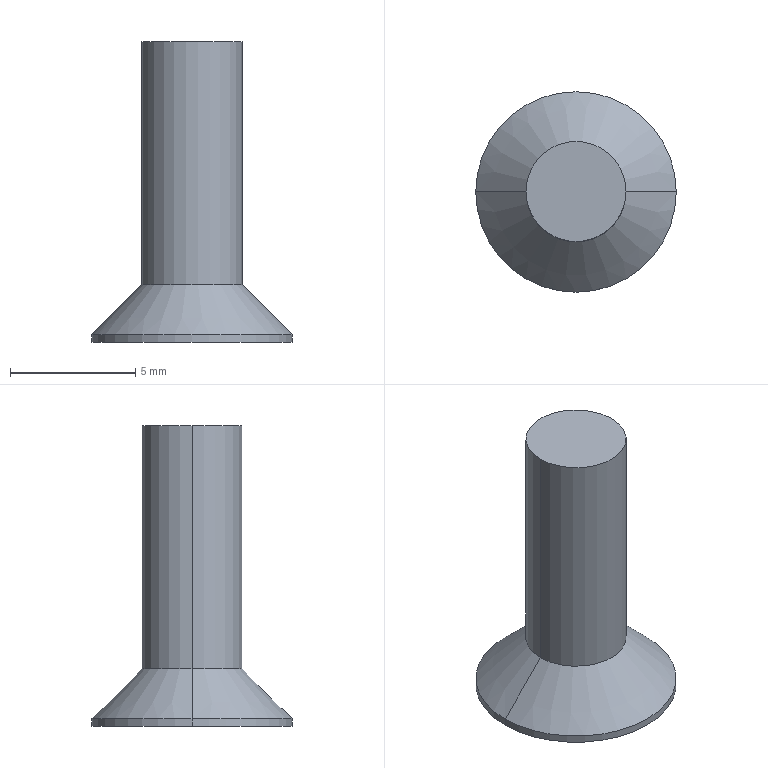Part | SolidWorks | features BaseBody 1, MoveFace 1 | 1 solid | 22 faces | box 8 x 8 x 12 mm | volume 187.399 mm3 | plane 14 | cone 4 | cylinder 4 | commonest cylinder face diameters 4 x2 8 x2
STEP:
#1=CARTESIAN_POINT('',(2.,0.,2.3));
#2=VERTEX_POINT('',#1);
#3=CARTESIAN_POINT('',(-2.,0.,2.3));
#4=VERTEX_POINT('',#3);
#5=CARTESIAN_POINT('',(0.,0.,2.3));
#6=DIRECTION('',(0.,0.,1.));
#7=DIRECTION('',(-1.,0.,0.));
#8=AXIS2_PLACEMENT_3D('',#5,#6,#7);
#9=CIRCLE('',#8,2.);
#10=EDGE_CURVE('',#2,#4,#9,.T.);
#11=ORIENTED_EDGE('',*,*,#10,.F.);
#12=CARTESIAN_POINT('',(4.,0.,0.3));
#13=VERTEX_POINT('',#12);
#14=CARTESIAN_POINT('',(4.,0.,0.3));
#15=DIRECTION('',(0.7071,0.,-0.7071));
#16=VECTOR('',#15,1000.);
#17=LINE('',#14,#16);
#18=EDGE_CURVE('',#2,#13,#17,.T.);
#19=ORIENTED_EDGE('',*,*,#18,.T.);
#20=CARTESIAN_POINT('',(-4.,0.,0.3));
#21=VERTEX_POINT('',#20);
#22=CARTESIAN_POINT('',(0.,0.,0.3));
#23=DIRECTION('',(0.,0.,1.));
#24=DIRECTION('',(-1.,0.,0.));
#25=AXIS2_PLACEMENT_3D('',#22,#23,#24);
#26=CIRCLE('',#25,4.);
#27=EDGE_CURVE('',#13,#21,#26,.T.);
#28=ORIENTED_EDGE('',*,*,#27,.T.);
#29=CARTESIAN_POINT('',(-4.,0.,0.3));
#30=DIRECTION('',(-0.7071,0.,-0.7071));
#31=VECTOR('',#30,1000.);
#32=LINE('',#29,#31);
#33=EDGE_CURVE('',#4,#21,#32,.T.);
#34=ORIENTED_EDGE('',*,*,#33,.F.);
#35=EDGE_LOOP('',(#11,#19,#28,#34));
#36=FACE_OUTER_BOUND('',#35,.T.);
#37=CARTESIAN_POINT('',(0.,0.,0.3));
#38=DIRECTION('',(0.,0.,-1.));
#39=DIRECTION('',(-1.,0.,0.));
#40=AXIS2_PLACEMENT_3D('',#37,#38,#39);
#41=CONICAL_SURFACE('',#40,4.,0.7854);
#42=ADVANCED_FACE('',(#36),#41,.T.);
#43=ORIENTED_EDGE('',*,*,#27,.F.);
#44=CARTESIAN_POINT('',(4.,0.,0.));
#45=VERTEX_POINT('',#44);
#46=CARTESIAN_POINT('',(4.,0.,2.3));
#47=DIRECTION('',(0.,0.,-1.));
#48=VECTOR('',#47,1000.);
#49=LINE('',#46,#48);
#50=EDGE_CURVE('',#13,#45,#49,.T.);
#51=ORIENTED_EDGE('',*,*,#50,.T.);
#52=CARTESIAN_POINT('',(-4.,0.,0.));
#53=VERTEX_POINT('',#52);
#54=CARTESIAN_POINT('',(0.,0.,0.));
#55=DIRECTION('',(0.,0.,1.));
#56=DIRECTION('',(-1.,0.,0.));
#57=AXIS2_PLACEMENT_3D('',#54,#55,#56);
#58=CIRCLE('',#57,4.);
#59=EDGE_CURVE('',#45,#53,#58,.T.);
#60=ORIENTED_EDGE('',*,*,#59,.T.);
#61=CARTESIAN_POINT('',(-4.,0.,2.3));
#62=DIRECTION('',(0.,0.,-1.));
#63=VECTOR('',#62,1000.);
#64=LINE('',#61,#63);
#65=EDGE_CURVE('',#21,#53,#64,.T.);
#66=ORIENTED_EDGE('',*,*,#65,.F.);
#67=EDGE_LOOP('',(#43,#51,#60,#66));
#68=FACE_OUTER_BOUND('',#67,.T.);
#69=CARTESIAN_POINT('',(0.,0.,2.3));
#70=DIRECTION('',(0.,0.,-1.));
#71=DIRECTION('',(-1.,0.,0.));
#72=AXIS2_PLACEMENT_3D('',#69,#70,#71);
#73=CYLINDRICAL_SURFACE('',#72,4.);
#74=ADVANCED_FACE('',(#68),#73,.T.);
#75=CARTESIAN_POINT('',(0.,0.,2.022));
#76=VERTEX_POINT('',#75);
#77=CARTESIAN_POINT('',(-1.25,0.,1.3));
#78=VERTEX_POINT('',#77);
#79=CARTESIAN_POINT('',(-1.25,0.,1.3));
#80=DIRECTION('',(-0.866,0.,-0.5));
#81=VECTOR('',#80,1000.);
#82=LINE('',#79,#81);
#83=EDGE_CURVE('',#76,#78,#82,.T.);
#84=ORIENTED_EDGE('',*,*,#83,.F.);
#85=CARTESIAN_POINT('',(1.25,0.,1.3));
#86=VERTEX_POINT('',#85);
#87=CARTESIAN_POINT('',(1.25,0.,1.3));
#88=DIRECTION('',(0.866,0.,-0.5));
#89=VECTOR('',#88,1000.);
#90=LINE('',#87,#89);
#91=EDGE_CURVE('',#76,#86,#90,.T.);
#92=ORIENTED_EDGE('',*,*,#91,.T.);
#93=CARTESIAN_POINT('',(1.083,-0.625,1.3));
#94=VERTEX_POINT('',#93);
#95=CARTESIAN_POINT('',(0.,0.,1.3));
#96=DIRECTION('',(0.,0.,1.));
#97=DIRECTION('',(-1.,0.,0.));
#98=AXIS2_PLACEMENT_3D('',#95,#96,#97);
#99=CIRCLE('',#98,1.25);
#100=EDGE_CURVE('',#94,#86,#99,.T.);
#101=ORIENTED_EDGE('',*,*,#100,.F.);
#102=CARTESIAN_POINT('',(0.,-1.25,1.3));
#103=VERTEX_POINT('',#102);
#104=CARTESIAN_POINT('',(0.,0.,1.3));
#105=DIRECTION('',(0.,0.,1.));
#106=DIRECTION('',(-1.,0.,0.));
#107=AXIS2_PLACEMENT_3D('',#104,#105,#106);
#108=CIRCLE('',#107,1.25);
#109=EDGE_CURVE('',#103,#94,#108,.T.);
#110=ORIENTED_EDGE('',*,*,#109,.F.);
#111=CARTESIAN_POINT('',(-1.083,-0.625,1.3));
#112=VERTEX_POINT('',#111);
#113=CARTESIAN_POINT('',(0.,0.,1.3));
#114=DIRECTION('',(0.,0.,1.));
#115=DIRECTION('',(-1.,0.,0.));
#116=AXIS2_PLACEMENT_3D('',#113,#114,#115);
#117=CIRCLE('',#116,1.25);
#118=EDGE_CURVE('',#112,#103,#117,.T.);
#119=ORIENTED_EDGE('',*,*,#118,.F.);
#120=CARTESIAN_POINT('',(0.,0.,1.3));
#121=DIRECTION('',(0.,0.,1.));
#122=DIRECTION('',(-1.,0.,0.));
#123=AXIS2_PLACEMENT_3D('',#120,#121,#122);
#124=CIRCLE('',#123,1.25);
#125=EDGE_CURVE('',#78,#112,#124,.T.);
#126=ORIENTED_EDGE('',*,*,#125,.F.);
#127=EDGE_LOOP('',(#84,#92,#101,#110,#119,#126));
#128=FACE_OUTER_BOUND('',#127,.T.);
#129=CARTESIAN_POINT('',(0.,0.,1.3));
#130=DIRECTION('',(0.,0.,-1.));
#131=DIRECTION('',(-1.,0.,0.));
#132=AXIS2_PLACEMENT_3D('',#129,#130,#131);
#133=CONICAL_SURFACE('',#132,1.25,1.047);
#134=ADVANCED_FACE('',(#128),#133,.F.);
#135=CARTESIAN_POINT('',(-2.,0.,12.));
#136=VERTEX_POINT('',#135);
#137=CARTESIAN_POINT('',(2.,0.,12.));
#138=VERTEX_POINT('',#137);
#139=CARTESIAN_POINT('',(0.,0.,12.));
#140=DIRECTION('',(0.,0.,-1.));
#141=DIRECTION('',(1.,0.,0.));
#142=AXIS2_PLACEMENT_3D('',#139,#140,#141);
#143=CIRCLE('',#142,2.);
#144=EDGE_CURVE('',#136,#138,#143,.T.);
#145=ORIENTED_EDGE('',*,*,#144,.T.);
#146=CARTESIAN_POINT('',(2.,0.,20.));
#147=DIRECTION('',(0.,0.,-1.));
#148=VECTOR('',#147,1000.);
#149=LINE('',#146,#148);
#150=EDGE_CURVE('',#138,#2,#149,.T.);
#151=ORIENTED_EDGE('',*,*,#150,.T.);
#152=ORIENTED_EDGE('',*,*,#10,.T.);
#153=CARTESIAN_POINT('',(-2.,0.,20.));
#154=DIRECTION('',(0.,0.,-1.));
#155=VECTOR('',#154,1000.);
#156=LINE('',#153,#155);
#157=EDGE_CURVE('',#136,#4,#156,.T.);
#158=ORIENTED_EDGE('',*,*,#157,.F.);
#159=EDGE_LOOP('',(#145,#151,#152,#158));
#160=FACE_OUTER_BOUND('',#159,.T.);
#161=CARTESIAN_POINT('',(0.,0.,20.));
#162=DIRECTION('',(0.,0.,-1.));
#163=DIRECTION('',(-1.,0.,0.));
#164=AXIS2_PLACEMENT_3D('',#161,#162,#163);
#165=CYLINDRICAL_SURFACE('',#164,2.);
#166=ADVANCED_FACE('',(#160),#165,.T.);
#167=ORIENTED_EDGE('',*,*,#150,.F.);
#168=CARTESIAN_POINT('',(0.,0.,12.));
#169=DIRECTION('',(0.,0.,-1.));
#170=DIRECTION('',(1.,0.,0.));
#171=AXIS2_PLACEMENT_3D('',#168,#169,#170);
#172=CIRCLE('',#171,2.);
#173=EDGE_CURVE('',#138,#136,#172,.T.);
#174=ORIENTED_EDGE('',*,*,#173,.T.);
#175=ORIENTED_EDGE('',*,*,#157,.T.);
#176=CARTESIAN_POINT('',(0.,0.,2.3));
#177=DIRECTION('',(0.,0.,1.));
#178=DIRECTION('',(-1.,0.,0.));
#179=AXIS2_PLACEMENT_3D('',#176,#177,#178);
#180=CIRCLE('',#179,2.);
#181=EDGE_CURVE('',#4,#2,#180,.T.);
#182=ORIENTED_EDGE('',*,*,#181,.T.);
#183=EDGE_LOOP('',(#167,#174,#175,#182));
#184=FACE_OUTER_BOUND('',#183,.T.);
#185=CARTESIAN_POINT('',(0.,0.,20.));
#186=DIRECTION('',(0.,0.,-1.));
#187=DIRECTION('',(-1.,0.,0.));
#188=AXIS2_PLACEMENT_3D('',#185,#186,#187);
#189=CYLINDRICAL_SURFACE('',#188,2.);
#190=ADVANCED_FACE('',(#184),#189,.T.);
#191=ORIENTED_EDGE('',*,*,#18,.F.);
#192=ORIENTED_EDGE('',*,*,#181,.F.);
#193=ORIENTED_EDGE('',*,*,#33,.T.);
#194=CARTESIAN_POINT('',(0.,0.,0.3));
#195=DIRECTION('',(0.,0.,1.));
#196=DIRECTION('',(-1.,0.,0.));
#197=AXIS2_PLACEMENT_3D('',#194,#195,#196);
#198=CIRCLE('',#197,4.);
#199=EDGE_CURVE('',#21,#13,#198,.T.);
#200=ORIENTED_EDGE('',*,*,#199,.T.);
#201=EDGE_LOOP('',(#191,#192,#193,#200));
#202=FACE_OUTER_BOUND('',#201,.T.);
#203=CARTESIAN_POINT('',(0.,0.,0.3));
#204=DIRECTION('',(0.,0.,-1.));
#205=DIRECTION('',(-1.,0.,0.));
#206=AXIS2_PLACEMENT_3D('',#203,#204,#205);
#207=CONICAL_SURFACE('',#206,4.,0.7854);
#208=ADVANCED_FACE('',(#202),#207,.T.);
#209=ORIENTED_EDGE('',*,*,#50,.F.);
#210=ORIENTED_EDGE('',*,*,#199,.F.);
#211=ORIENTED_EDGE('',*,*,#65,.T.);
#212=CARTESIAN_POINT('',(0.,0.,0.));
#213=DIRECTION('',(0.,0.,1.));
#214=DIRECTION('',(-1.,0.,0.));
#215=AXIS2_PLACEMENT_3D('',#212,#213,#214);
#216=CIRCLE('',#215,4.);
#217=EDGE_CURVE('',#53,#45,#216,.T.);
#218=ORIENTED_EDGE('',*,*,#217,.T.);
#219=EDGE_LOOP('',(#209,#210,#211,#218));
#220=FACE_OUTER_BOUND('',#219,.T.);
#221=CARTESIAN_POINT('',(0.,0.,2.3));
#222=DIRECTION('',(0.,0.,-1.));
#223=DIRECTION('',(-1.,0.,0.));
#224=AXIS2_PLACEMENT_3D('',#221,#222,#223);
#225=CYLINDRICAL_SURFACE('',#224,4.);
#226=ADVANCED_FACE('',(#220),#225,.T.);
#227=ORIENTED_EDGE('',*,*,#144,.F.);
#228=ORIENTED_EDGE('',*,*,#173,.F.);
#229=EDGE_LOOP('',(#227,#228));
#230=FACE_OUTER_BOUND('',#229,.T.);
#231=CARTESIAN_POINT('',(0.,0.,12.));
#232=DIRECTION('',(0.,0.,1.));
#233=DIRECTION('',(1.,0.,0.));
#234=AXIS2_PLACEMENT_3D('',#231,#232,#233);
#235=PLANE('',#234);
#236=ADVANCED_FACE('',(#230),#235,.T.);
#237=ORIENTED_EDGE('',*,*,#217,.F.);
#238=ORIENTED_EDGE('',*,*,#59,.F.);
#239=EDGE_LOOP('',(#237,#238));
#240=FACE_OUTER_BOUND('',#239,.T.);
#241=CARTESIAN_POINT('',(-1.443,0.,0.));
#242=VERTEX_POINT('',#241);
#243=CARTESIAN_POINT('',(-0.7217,1.25,0.));
#244=VERTEX_POINT('',#243);
#245=CARTESIAN_POINT('',(-1.443,0.,0.));
#246=DIRECTION('',(0.5,0.866,0.));
#247=VECTOR('',#246,1000.);
#248=LINE('',#245,#247);
#249=EDGE_CURVE('',#242,#244,#248,.T.);
#250=ORIENTED_EDGE('',*,*,#249,.F.);
#251=CARTESIAN_POINT('',(-0.7217,-1.25,0.));
#252=VERTEX_POINT('',#251);
#253=CARTESIAN_POINT('',(-0.7217,-1.25,0.));
#254=DIRECTION('',(-0.5,0.866,0.));
#255=VECTOR('',#254,1000.);
#256=LINE('',#253,#255);
#257=EDGE_CURVE('',#252,#242,#256,.T.);
#258=ORIENTED_EDGE('',*,*,#257,.F.);
#259=CARTESIAN_POINT('',(0.7217,-1.25,0.));
#260=VERTEX_POINT('',#259);
#261=CARTESIAN_POINT('',(0.,-1.25,0.));
#262=DIRECTION('',(-1.,0.,0.));
#263=VECTOR('',#262,1000.);
#264=LINE('',#261,#263);
#265=EDGE_CURVE('',#260,#252,#264,.T.);
#266=ORIENTED_EDGE('',*,*,#265,.F.);
#267=CARTESIAN_POINT('',(1.443,0.,0.));
#268=VERTEX_POINT('',#267);
#269=CARTESIAN_POINT('',(1.443,0.,0.));
#270=DIRECTION('',(-0.5,-0.866,0.));
#271=VECTOR('',#270,1000.);
#272=LINE('',#269,#271);
#273=EDGE_CURVE('',#268,#260,#272,.T.);
#274=ORIENTED_EDGE('',*,*,#273,.F.);
#275=CARTESIAN_POINT('',(0.7217,1.25,0.));
#276=VERTEX_POINT('',#275);
#277=CARTESIAN_POINT('',(0.7217,1.25,0.));
#278=DIRECTION('',(0.5,-0.866,0.));
#279=VECTOR('',#278,1000.);
#280=LINE('',#277,#279);
#281=EDGE_CURVE('',#276,#268,#280,.T.);
#282=ORIENTED_EDGE('',*,*,#281,.F.);
#283=CARTESIAN_POINT('',(0.,1.25,0.));
#284=DIRECTION('',(1.,0.,0.));
#285=VECTOR('',#284,1000.);
#286=LINE('',#283,#285);
#287=EDGE_CURVE('',#244,#276,#286,.T.);
#288=ORIENTED_EDGE('',*,*,#287,.F.);
#289=EDGE_LOOP('',(#250,#258,#266,#274,#282,#288));
#290=FACE_BOUND('',#289,.T.);
#291=CARTESIAN_POINT('',(0.,0.,0.));
#292=DIRECTION('',(0.,0.,1.));
#293=DIRECTION('',(1.,0.,0.));
#294=AXIS2_PLACEMENT_3D('',#291,#292,#293);
#295=PLANE('',#294);
#296=ADVANCED_FACE('',(#240,#290),#295,.F.);
#297=CARTESIAN_POINT('',(0.7217,1.25,1.3));
#298=VERTEX_POINT('',#297);
#299=CARTESIAN_POINT('',(0.7217,1.25,1.3));
#300=DIRECTION('',(0.,0.,-1.));
#301=VECTOR('',#300,1000.);
#302=LINE('',#299,#301);
#303=EDGE_CURVE('',#298,#276,#302,.T.);
#304=ORIENTED_EDGE('',*,*,#303,.F.);
#305=CARTESIAN_POINT('',(0.,1.25,1.3));
#306=VERTEX_POINT('',#305);
#307=CARTESIAN_POINT('',(-0.7217,1.25,1.3));
#308=DIRECTION('',(1.,0.,0.));
#309=VECTOR('',#308,1000.);
#310=LINE('',#307,#309);
#311=EDGE_CURVE('',#306,#298,#310,.T.);
#312=ORIENTED_EDGE('',*,*,#311,.F.);
#313=CARTESIAN_POINT('',(-0.7217,1.25,1.3));
#314=VERTEX_POINT('',#313);
#315=CARTESIAN_POINT('',(-0.7217,1.25,1.3));
#316=DIRECTION('',(1.,0.,0.));
#317=VECTOR('',#316,1000.);
#318=LINE('',#315,#317);
#319=EDGE_CURVE('',#314,#306,#318,.T.);
#320=ORIENTED_EDGE('',*,*,#319,.F.);
#321=CARTESIAN_POINT('',(-0.7217,1.25,1.3));
#322=DIRECTION('',(0.,0.,1.));
#323=VECTOR('',#322,1000.);
#324=LINE('',#321,#323);
#325=EDGE_CURVE('',#244,#314,#324,.T.);
#326=ORIENTED_EDGE('',*,*,#325,.F.);
#327=ORIENTED_EDGE('',*,*,#287,.T.);
#328=EDGE_LOOP('',(#304,#312,#320,#326,#327));
#329=FACE_OUTER_BOUND('',#328,.T.);
#330=CARTESIAN_POINT('',(-0.7217,1.25,1.3));
#331=DIRECTION('',(0.,1.,0.));
#332=DIRECTION('',(0.,0.,1.));
#333=AXIS2_PLACEMENT_3D('',#330,#331,#332);
#334=PLANE('',#333);
#335=ADVANCED_FACE('',(#329),#334,.F.);
#336=ORIENTED_EDGE('',*,*,#325,.T.);
#337=CARTESIAN_POINT('',(-1.083,0.625,1.3));
#338=VERTEX_POINT('',#337);
#339=CARTESIAN_POINT('',(-1.443,0.,1.3));
#340=DIRECTION('',(0.5,0.866,0.));
#341=VECTOR('',#340,1000.);
#342=LINE('',#339,#341);
#343=EDGE_CURVE('',#338,#314,#342,.T.);
#344=ORIENTED_EDGE('',*,*,#343,.F.);
#345=CARTESIAN_POINT('',(-1.443,0.,1.3));
#346=VERTEX_POINT('',#345);
#347=CARTESIAN_POINT('',(-1.443,0.,1.3));
#348=DIRECTION('',(0.5,0.866,0.));
#349=VECTOR('',#348,1000.);
#350=LINE('',#347,#349);
#351=EDGE_CURVE('',#346,#338,#350,.T.);
#352=ORIENTED_EDGE('',*,*,#351,.F.);
#353=CARTESIAN_POINT('',(-1.443,0.,1.3));
#354=DIRECTION('',(0.,0.,1.));
#355=VECTOR('',#354,1000.);
#356=LINE('',#353,#355);
#357=EDGE_CURVE('',#242,#346,#356,.T.);
#358=ORIENTED_EDGE('',*,*,#357,.F.);
#359=ORIENTED_EDGE('',*,*,#249,.T.);
#360=EDGE_LOOP('',(#336,#344,#352,#358,#359));
#361=FACE_OUTER_BOUND('',#360,.T.);
#362=CARTESIAN_POINT('',(-1.443,0.,1.3));
#363=DIRECTION('',(-0.866,0.5,0.));
#364=DIRECTION('',(-0.5,-0.866,0.));
#365=AXIS2_PLACEMENT_3D('',#362,#363,#364);
#366=PLANE('',#365);
#367=ADVANCED_FACE('',(#361),#366,.F.);
#368=ORIENTED_EDGE('',*,*,#357,.T.);
#369=CARTESIAN_POINT('',(-0.7217,-1.25,1.3));
#370=DIRECTION('',(-0.5,0.866,0.));
#371=VECTOR('',#370,1000.);
#372=LINE('',#369,#371);
#373=EDGE_CURVE('',#112,#346,#372,.T.);
#374=ORIENTED_EDGE('',*,*,#373,.F.);
#375=CARTESIAN_POINT('',(-0.7217,-1.25,1.3));
#376=VERTEX_POINT('',#375);
#377=CARTESIAN_POINT('',(-0.7217,-1.25,1.3));
#378=DIRECTION('',(-0.5,0.866,0.));
#379=VECTOR('',#378,1000.);
#380=LINE('',#377,#379);
#381=EDGE_CURVE('',#376,#112,#380,.T.);
#382=ORIENTED_EDGE('',*,*,#381,.F.);
#383=CARTESIAN_POINT('',(-0.7217,-1.25,1.3));
#384=DIRECTION('',(0.,0.,1.));
#385=VECTOR('',#384,1000.);
#386=LINE('',#383,#385);
#387=EDGE_CURVE('',#252,#376,#386,.T.);
#388=ORIENTED_EDGE('',*,*,#387,.F.);
#389=ORIENTED_EDGE('',*,*,#257,.T.);
#390=EDGE_LOOP('',(#368,#374,#382,#388,#389));
#391=FACE_OUTER_BOUND('',#390,.T.);
#392=CARTESIAN_POINT('',(-0.7217,-1.25,1.3));
#393=DIRECTION('',(-0.866,-0.5,0.));
#394=DIRECTION('',(0.5,-0.866,0.));
#395=AXIS2_PLACEMENT_3D('',#392,#393,#394);
#396=PLANE('',#395);
#397=ADVANCED_FACE('',(#391),#396,.F.);
#398=ORIENTED_EDGE('',*,*,#387,.T.);
#399=CARTESIAN_POINT('',(0.7217,-1.25,1.3));
#400=DIRECTION('',(-1.,0.,0.));
#401=VECTOR('',#400,1000.);
#402=LINE('',#399,#401);
#403=EDGE_CURVE('',#103,#376,#402,.T.);
#404=ORIENTED_EDGE('',*,*,#403,.F.);
#405=CARTESIAN_POINT('',(0.7217,-1.25,1.3));
#406=VERTEX_POINT('',#405);
#407=CARTESIAN_POINT('',(0.7217,-1.25,1.3));
#408=DIRECTION('',(-1.,0.,0.));
#409=VECTOR('',#408,1000.);
#410=LINE('',#407,#409);
#411=EDGE_CURVE('',#406,#103,#410,.T.);
#412=ORIENTED_EDGE('',*,*,#411,.F.);
#413=CARTESIAN_POINT('',(0.7217,-1.25,1.3));
#414=DIRECTION('',(0.,0.,1.));
#415=VECTOR('',#414,1000.);
#416=LINE('',#413,#415);
#417=EDGE_CURVE('',#260,#406,#416,.T.);
#418=ORIENTED_EDGE('',*,*,#417,.F.);
#419=ORIENTED_EDGE('',*,*,#265,.T.);
#420=EDGE_LOOP('',(#398,#404,#412,#418,#419));
#421=FACE_OUTER_BOUND('',#420,.T.);
#422=CARTESIAN_POINT('',(0.7217,-1.25,1.3));
#423=DIRECTION('',(0.,-1.,0.));
#424=DIRECTION('',(0.,0.,-1.));
#425=AXIS2_PLACEMENT_3D('',#422,#423,#424);
#426=PLANE('',#425);
#427=ADVANCED_FACE('',(#421),#426,.F.);
#428=ORIENTED_EDGE('',*,*,#417,.T.);
#429=CARTESIAN_POINT('',(1.443,0.,1.3));
#430=DIRECTION('',(-0.5,-0.866,0.));
#431=VECTOR('',#430,1000.);
#432=LINE('',#429,#431);
#433=EDGE_CURVE('',#94,#406,#432,.T.);
#434=ORIENTED_EDGE('',*,*,#433,.F.);
#435=CARTESIAN_POINT('',(1.443,0.,1.3));
#436=VERTEX_POINT('',#435);
#437=CARTESIAN_POINT('',(1.443,0.,1.3));
#438=DIRECTION('',(-0.5,-0.866,0.));
#439=VECTOR('',#438,1000.);
#440=LINE('',#437,#439);
#441=EDGE_CURVE('',#436,#94,#440,.T.);
#442=ORIENTED_EDGE('',*,*,#441,.F.);
#443=CARTESIAN_POINT('',(1.443,0.,1.3));
#444=DIRECTION('',(0.,0.,1.));
#445=VECTOR('',#444,1000.);
#446=LINE('',#443,#445);
#447=EDGE_CURVE('',#268,#436,#446,.T.);
#448=ORIENTED_EDGE('',*,*,#447,.F.);
#449=ORIENTED_EDGE('',*,*,#273,.T.);
#450=EDGE_LOOP('',(#428,#434,#442,#448,#449));
#451=FACE_OUTER_BOUND('',#450,.T.);
#452=CARTESIAN_POINT('',(1.443,0.,1.3));
#453=DIRECTION('',(0.866,-0.5,0.));
#454=DIRECTION('',(0.5,0.866,0.));
#455=AXIS2_PLACEMENT_3D('',#452,#453,#454);
#456=PLANE('',#455);
#457=ADVANCED_FACE('',(#451),#456,.F.);
#458=ORIENTED_EDGE('',*,*,#447,.T.);
#459=CARTESIAN_POINT('',(1.083,0.625,1.3));
#460=VERTEX_POINT('',#459);
#461=CARTESIAN_POINT('',(0.7217,1.25,1.3));
#462=DIRECTION('',(0.5,-0.866,0.));
#463=VECTOR('',#462,1000.);
#464=LINE('',#461,#463);
#465=EDGE_CURVE('',#460,#436,#464,.T.);
#466=ORIENTED_EDGE('',*,*,#465,.F.);
#467=CARTESIAN_POINT('',(0.7217,1.25,1.3));
#468=DIRECTION('',(0.5,-0.866,0.));
#469=VECTOR('',#468,1000.);
#470=LINE('',#467,#469);
#471=EDGE_CURVE('',#298,#460,#470,.T.);
#472=ORIENTED_EDGE('',*,*,#471,.F.);
#473=ORIENTED_EDGE('',*,*,#303,.T.);
#474=ORIENTED_EDGE('',*,*,#281,.T.);
#475=EDGE_LOOP('',(#458,#466,#472,#473,#474));
#476=FACE_OUTER_BOUND('',#475,.T.);
#477=CARTESIAN_POINT('',(0.7217,1.25,1.3));
#478=DIRECTION('',(0.866,0.5,0.));
#479=DIRECTION('',(-0.5,0.866,0.));
#480=AXIS2_PLACEMENT_3D('',#477,#478,#479);
#481=PLANE('',#480);
#482=ADVANCED_FACE('',(#476),#481,.F.);
#483=ORIENTED_EDGE('',*,*,#311,.T.);
#484=ORIENTED_EDGE('',*,*,#471,.T.);
#485=CARTESIAN_POINT('',(0.,0.,1.3));
#486=DIRECTION('',(0.,0.,1.));
#487=DIRECTION('',(-1.,0.,0.));
#488=AXIS2_PLACEMENT_3D('',#485,#486,#487);
#489=CIRCLE('',#488,1.25);
#490=EDGE_CURVE('',#460,#306,#489,.T.);
#491=ORIENTED_EDGE('',*,*,#490,.T.);
#492=EDGE_LOOP('',(#483,#484,#491));
#493=FACE_OUTER_BOUND('',#492,.T.);
#494=CARTESIAN_POINT('',(0.,0.,1.3));
#495=DIRECTION('',(0.,0.,-1.));
#496=DIRECTION('',(-1.,0.,0.));
#497=AXIS2_PLACEMENT_3D('',#494,#495,#496);
#498=PLANE('',#497);
#499=ADVANCED_FACE('',(#493),#498,.T.);
#500=ORIENTED_EDGE('',*,*,#343,.T.);
#501=ORIENTED_EDGE('',*,*,#319,.T.);
#502=CARTESIAN_POINT('',(0.,0.,1.3));
#503=DIRECTION('',(0.,0.,1.));
#504=DIRECTION('',(-1.,0.,0.));
#505=AXIS2_PLACEMENT_3D('',#502,#503,#504);
#506=CIRCLE('',#505,1.25);
#507=EDGE_CURVE('',#306,#338,#506,.T.);
#508=ORIENTED_EDGE('',*,*,#507,.T.);
#509=EDGE_LOOP('',(#500,#501,#508));
#510=FACE_OUTER_BOUND('',#509,.T.);
#511=CARTESIAN_POINT('',(0.,0.,1.3));
#512=DIRECTION('',(0.,0.,-1.));
#513=DIRECTION('',(-1.,0.,0.));
#514=AXIS2_PLACEMENT_3D('',#511,#512,#513);
#515=PLANE('',#514);
#516=ADVANCED_FACE('',(#510),#515,.T.);
#517=ORIENTED_EDGE('',*,*,#351,.T.);
#518=CARTESIAN_POINT('',(0.,0.,1.3));
#519=DIRECTION('',(0.,0.,1.));
#520=DIRECTION('',(-1.,0.,0.));
#521=AXIS2_PLACEMENT_3D('',#518,#519,#520);
#522=CIRCLE('',#521,1.25);
#523=EDGE_CURVE('',#338,#78,#522,.T.);
#524=ORIENTED_EDGE('',*,*,#523,.T.);
#525=ORIENTED_EDGE('',*,*,#125,.T.);
#526=ORIENTED_EDGE('',*,*,#373,.T.);
#527=EDGE_LOOP('',(#517,#524,#525,#526));
#528=FACE_OUTER_BOUND('',#527,.T.);
#529=CARTESIAN_POINT('',(0.,0.,1.3));
#530=DIRECTION('',(0.,0.,-1.));
#531=DIRECTION('',(-1.,0.,0.));
#532=AXIS2_PLACEMENT_3D('',#529,#530,#531);
#533=PLANE('',#532);
#534=ADVANCED_FACE('',(#528),#533,.T.);
#535=ORIENTED_EDGE('',*,*,#403,.T.);
#536=ORIENTED_EDGE('',*,*,#381,.T.);
#537=ORIENTED_EDGE('',*,*,#118,.T.);
#538=EDGE_LOOP('',(#535,#536,#537));
#539=FACE_OUTER_BOUND('',#538,.T.);
#540=CARTESIAN_POINT('',(0.,0.,1.3));
#541=DIRECTION('',(0.,0.,-1.));
#542=DIRECTION('',(-1.,0.,0.));
#543=AXIS2_PLACEMENT_3D('',#540,#541,#542);
#544=PLANE('',#543);
#545=ADVANCED_FACE('',(#539),#544,.T.);
#546=ORIENTED_EDGE('',*,*,#433,.T.);
#547=ORIENTED_EDGE('',*,*,#411,.T.);
#548=ORIENTED_EDGE('',*,*,#109,.T.);
#549=EDGE_LOOP('',(#546,#547,#548));
#550=FACE_OUTER_BOUND('',#549,.T.);
#551=CARTESIAN_POINT('',(0.,0.,1.3));
#552=DIRECTION('',(0.,0.,-1.));
#553=DIRECTION('',(-1.,0.,0.));
#554=AXIS2_PLACEMENT_3D('',#551,#552,#553);
#555=PLANE('',#554);
#556=ADVANCED_FACE('',(#550),#555,.T.);
#557=ORIENTED_EDGE('',*,*,#441,.T.);
#558=ORIENTED_EDGE('',*,*,#100,.T.);
#559=CARTESIAN_POINT('',(0.,0.,1.3));
#560=DIRECTION('',(0.,0.,1.));
#561=DIRECTION('',(-1.,0.,0.));
#562=AXIS2_PLACEMENT_3D('',#559,#560,#561);
#563=CIRCLE('',#562,1.25);
#564=EDGE_CURVE('',#86,#460,#563,.T.);
#565=ORIENTED_EDGE('',*,*,#564,.T.);
#566=ORIENTED_EDGE('',*,*,#465,.T.);
#567=EDGE_LOOP('',(#557,#558,#565,#566));
#568=FACE_OUTER_BOUND('',#567,.T.);
#569=CARTESIAN_POINT('',(0.,0.,1.3));
#570=DIRECTION('',(0.,0.,-1.));
#571=DIRECTION('',(-1.,0.,0.));
#572=AXIS2_PLACEMENT_3D('',#569,#570,#571);
#573=PLANE('',#572);
#574=ADVANCED_FACE('',(#568),#573,.T.);
#575=ORIENTED_EDGE('',*,*,#91,.F.);
#576=ORIENTED_EDGE('',*,*,#83,.T.);
#577=ORIENTED_EDGE('',*,*,#523,.F.);
#578=ORIENTED_EDGE('',*,*,#507,.F.);
#579=ORIENTED_EDGE('',*,*,#490,.F.);
#580=ORIENTED_EDGE('',*,*,#564,.F.);
#581=EDGE_LOOP('',(#575,#576,#577,#578,#579,#580));
#582=FACE_OUTER_BOUND('',#581,.T.);
#583=CARTESIAN_POINT('',(0.,0.,1.3));
#584=DIRECTION('',(0.,0.,-1.));
#585=DIRECTION('',(-1.,0.,0.));
#586=AXIS2_PLACEMENT_3D('',#583,#584,#585);
#587=CONICAL_SURFACE('',#586,1.25,1.047);
#588=ADVANCED_FACE('',(#582),#587,.F.);
#589=CLOSED_SHELL('',(#42,#74,#134,#166,#190,#208,#226,#236,#296,#335,#367,#397,#427,#457,#482,#499,#516,#534,#545,#556,#574,#588));
#590=MANIFOLD_SOLID_BREP('',#589);
#591=CARTESIAN_POINT('',(0.,0.,0.));
#592=DIRECTION('',(0.,0.,1.));
#593=DIRECTION('',(1.,0.,0.));
#594=AXIS2_PLACEMENT_3D('',#591,#592,#593);
#595=(LENGTH_UNIT()NAMED_UNIT(*)SI_UNIT(.MILLI.,.METRE.));
#596=UNCERTAINTY_MEASURE_WITH_UNIT(LENGTH_MEASURE(0.00001),#595,'','');
#597=(NAMED_UNIT(*)PLANE_ANGLE_UNIT()SI_UNIT($,.RADIAN.));
#598=(NAMED_UNIT(*)SI_UNIT($,.STERADIAN.)SOLID_ANGLE_UNIT());
#599=(GEOMETRIC_REPRESENTATION_CONTEXT(3)GLOBAL_UNCERTAINTY_ASSIGNED_CONTEXT((#596))GLOBAL_UNIT_ASSIGNED_CONTEXT((#595,#597,#598))REPRESENTATION_CONTEXT('',''));
#600=ADVANCED_BREP_SHAPE_REPRESENTATION('',(#590,#594),#599);